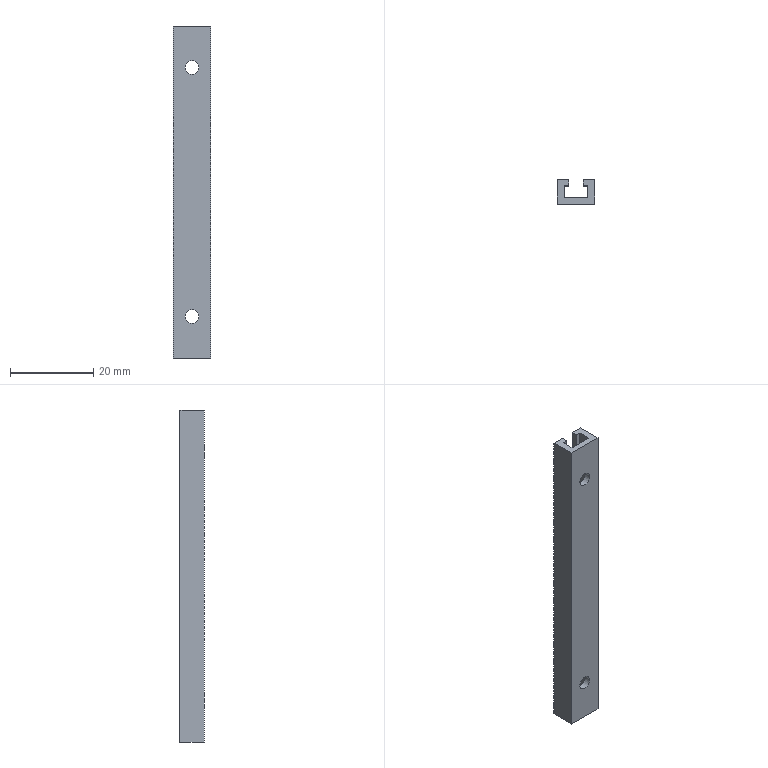Part | NX | 1 solid | 913 faces | box 9 x 6 x 80 mm | volume 2485 mm3 | plane 819 | spline 88 | cylinder 6 | commonest cylinder face diameters 6 x4 3.3 x2